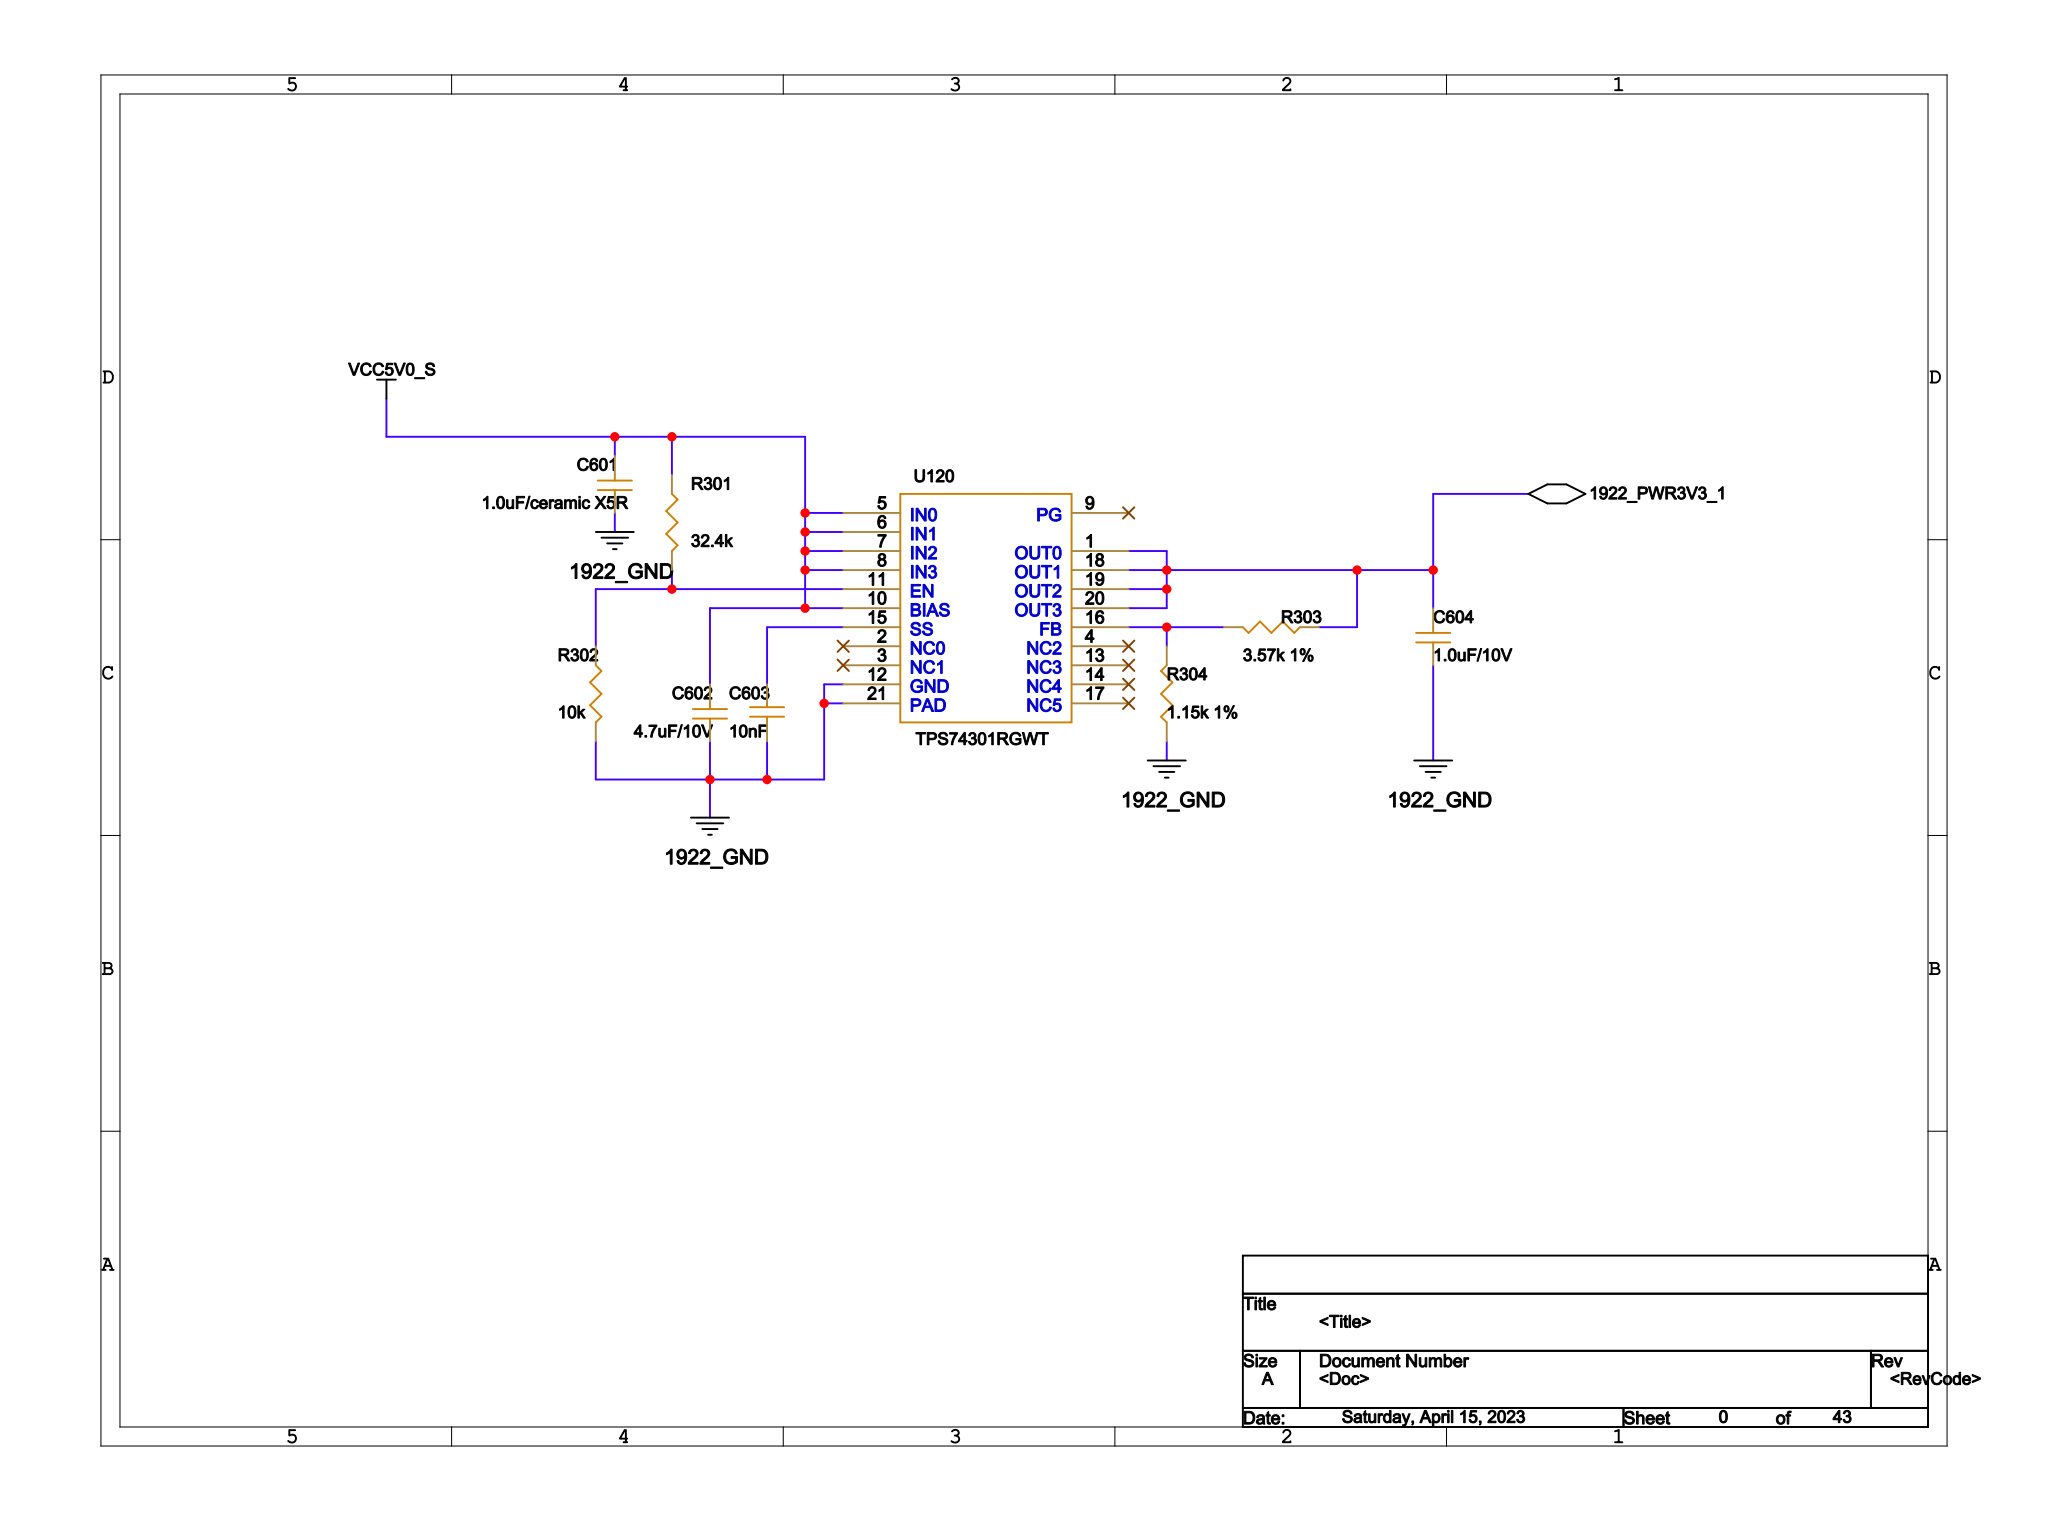Circuit board | Cadence Allegro | 1034 parts | 912 nets | one sheet of the schematic
Parts on this sheet (reference | value | footprint):
C601 | 1.0uF/ceramic X5R | C0402
C602 | 4.7uF/10V | C0402
C603 | 10nF | C0402
C604 | 1.0uF/10V | C0402
R301 | 32.4k | R0402
R302 | 10k | R0402
R303 | 3.57k 1% | R0402
R304 | 1.15k 1% | R0402
U120 | TPS74301RGWT | TPS74301_VQFN
Nets of these parts (net: part-pin ...):
VCC5V0_S: C601-2 C602-2 R301-1 U120-5 U120-6 U120-7 U120-8 U120-10
1922_GND: C601-1 C602-1 C603-2 C604-1 R302-2 R304-1 U120-12 U120-21
PWR1922_3V3_1: C604-2 R303-1 U120-1 U120-18 U120-19 U120-20
N14251186: C603-1 U120-15
N14251098: R301-2 R302-1 U120-11
N14251194: R303-2 R304-2 U120-16